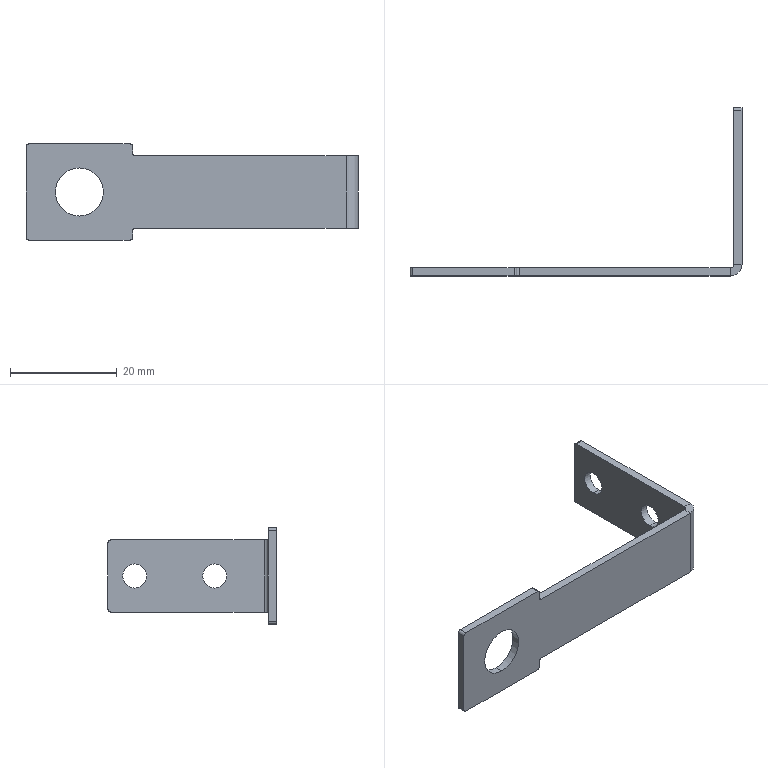Part | STEP file | PN_0011 (default) | 1 solid | 32 faces | box 62.237 x 31.5 x 18 mm | volume 1846 mm3 | cylinder 16 | plane 16 | commonest cylinder face diameters 1 x8 4.5 x4 9 x2 1.473 x1 4.473 x1